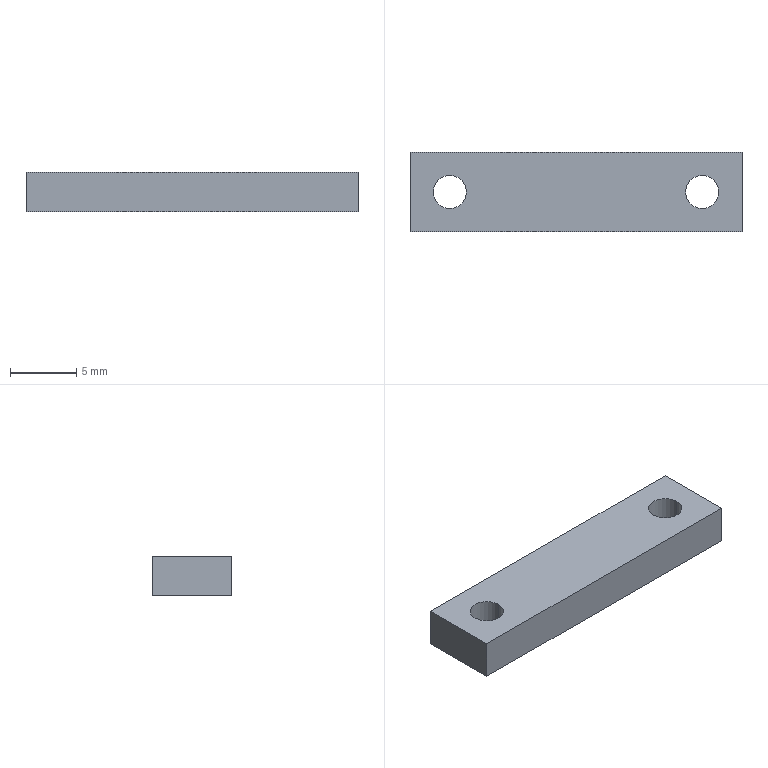Part | STEP file | 866-BDO024-93-11A | 1 solid | 10 faces | box 25 x 6 x 3 mm | volume 420.548 mm3 | plane 6 | cylinder 4 | commonest cylinder face diameters 2.5 x4
STEP:
#1=CARTESIAN_POINT('',(-10.75,0.,0.));
#2=VERTEX_POINT('',#1);
#3=CARTESIAN_POINT('',(-8.25,0.,0.));
#4=VERTEX_POINT('',#3);
#5=CARTESIAN_POINT('',(-9.5,0.,0.));
#6=DIRECTION('',(0.,0.,1.));
#7=DIRECTION('',(1.,0.,0.));
#8=AXIS2_PLACEMENT_3D('',#5,#6,#7);
#9=CIRCLE('',#8,1.25);
#10=EDGE_CURVE('',#2,#4,#9,.T.);
#11=ORIENTED_EDGE('',*,*,#10,.F.);
#12=CARTESIAN_POINT('',(-10.75,0.,3.));
#13=VERTEX_POINT('',#12);
#14=CARTESIAN_POINT('',(-10.75,0.,3.));
#15=DIRECTION('',(0.,0.,1.));
#16=VECTOR('',#15,1000.);
#17=LINE('',#14,#16);
#18=EDGE_CURVE('',#2,#13,#17,.T.);
#19=ORIENTED_EDGE('',*,*,#18,.T.);
#20=CARTESIAN_POINT('',(-8.25,0.,3.));
#21=VERTEX_POINT('',#20);
#22=CARTESIAN_POINT('',(-9.5,0.,3.));
#23=DIRECTION('',(0.,0.,1.));
#24=DIRECTION('',(1.,0.,0.));
#25=AXIS2_PLACEMENT_3D('',#22,#23,#24);
#26=CIRCLE('',#25,1.25);
#27=EDGE_CURVE('',#13,#21,#26,.T.);
#28=ORIENTED_EDGE('',*,*,#27,.T.);
#29=CARTESIAN_POINT('',(-8.25,0.,3.));
#30=DIRECTION('',(0.,0.,1.));
#31=VECTOR('',#30,1000.);
#32=LINE('',#29,#31);
#33=EDGE_CURVE('',#4,#21,#32,.T.);
#34=ORIENTED_EDGE('',*,*,#33,.F.);
#35=EDGE_LOOP('',(#11,#19,#28,#34));
#36=FACE_OUTER_BOUND('',#35,.T.);
#37=CARTESIAN_POINT('',(-9.5,0.,3.));
#38=DIRECTION('',(0.,0.,1.));
#39=DIRECTION('',(1.,0.,0.));
#40=AXIS2_PLACEMENT_3D('',#37,#38,#39);
#41=CYLINDRICAL_SURFACE('',#40,1.25);
#42=ADVANCED_FACE('',(#36),#41,.F.);
#43=CARTESIAN_POINT('',(8.25,0.,0.));
#44=VERTEX_POINT('',#43);
#45=CARTESIAN_POINT('',(10.75,0.,0.));
#46=VERTEX_POINT('',#45);
#47=CARTESIAN_POINT('',(9.5,0.,0.));
#48=DIRECTION('',(0.,0.,1.));
#49=DIRECTION('',(1.,0.,0.));
#50=AXIS2_PLACEMENT_3D('',#47,#48,#49);
#51=CIRCLE('',#50,1.25);
#52=EDGE_CURVE('',#44,#46,#51,.T.);
#53=ORIENTED_EDGE('',*,*,#52,.F.);
#54=CARTESIAN_POINT('',(8.25,0.,3.));
#55=VERTEX_POINT('',#54);
#56=CARTESIAN_POINT('',(8.25,0.,3.));
#57=DIRECTION('',(0.,0.,1.));
#58=VECTOR('',#57,1000.);
#59=LINE('',#56,#58);
#60=EDGE_CURVE('',#44,#55,#59,.T.);
#61=ORIENTED_EDGE('',*,*,#60,.T.);
#62=CARTESIAN_POINT('',(10.75,0.,3.));
#63=VERTEX_POINT('',#62);
#64=CARTESIAN_POINT('',(9.5,0.,3.));
#65=DIRECTION('',(0.,0.,1.));
#66=DIRECTION('',(1.,0.,0.));
#67=AXIS2_PLACEMENT_3D('',#64,#65,#66);
#68=CIRCLE('',#67,1.25);
#69=EDGE_CURVE('',#55,#63,#68,.T.);
#70=ORIENTED_EDGE('',*,*,#69,.T.);
#71=CARTESIAN_POINT('',(10.75,0.,3.));
#72=DIRECTION('',(0.,0.,1.));
#73=VECTOR('',#72,1000.);
#74=LINE('',#71,#73);
#75=EDGE_CURVE('',#46,#63,#74,.T.);
#76=ORIENTED_EDGE('',*,*,#75,.F.);
#77=EDGE_LOOP('',(#53,#61,#70,#76));
#78=FACE_OUTER_BOUND('',#77,.T.);
#79=CARTESIAN_POINT('',(9.5,0.,3.));
#80=DIRECTION('',(0.,0.,1.));
#81=DIRECTION('',(1.,0.,0.));
#82=AXIS2_PLACEMENT_3D('',#79,#80,#81);
#83=CYLINDRICAL_SURFACE('',#82,1.25);
#84=ADVANCED_FACE('',(#78),#83,.F.);
#85=CARTESIAN_POINT('',(-9.5,0.,3.));
#86=DIRECTION('',(0.,0.,1.));
#87=DIRECTION('',(1.,0.,0.));
#88=AXIS2_PLACEMENT_3D('',#85,#86,#87);
#89=CIRCLE('',#88,1.25);
#90=EDGE_CURVE('',#21,#13,#89,.T.);
#91=ORIENTED_EDGE('',*,*,#90,.F.);
#92=ORIENTED_EDGE('',*,*,#27,.F.);
#93=EDGE_LOOP('',(#91,#92));
#94=FACE_BOUND('',#93,.T.);
#95=CARTESIAN_POINT('',(12.5,-3.,3.));
#96=VERTEX_POINT('',#95);
#97=CARTESIAN_POINT('',(-12.5,-3.,3.));
#98=VERTEX_POINT('',#97);
#99=CARTESIAN_POINT('',(-12.5,-3.,3.));
#100=DIRECTION('',(-1.,0.,0.));
#101=VECTOR('',#100,1000.);
#102=LINE('',#99,#101);
#103=EDGE_CURVE('',#96,#98,#102,.T.);
#104=ORIENTED_EDGE('',*,*,#103,.F.);
#105=CARTESIAN_POINT('',(12.5,3.,3.));
#106=VERTEX_POINT('',#105);
#107=CARTESIAN_POINT('',(12.5,3.,3.));
#108=DIRECTION('',(0.,-1.,0.));
#109=VECTOR('',#108,1000.);
#110=LINE('',#107,#109);
#111=EDGE_CURVE('',#106,#96,#110,.T.);
#112=ORIENTED_EDGE('',*,*,#111,.F.);
#113=CARTESIAN_POINT('',(-12.5,3.,3.));
#114=VERTEX_POINT('',#113);
#115=CARTESIAN_POINT('',(-12.5,3.,3.));
#116=DIRECTION('',(1.,0.,0.));
#117=VECTOR('',#116,1000.);
#118=LINE('',#115,#117);
#119=EDGE_CURVE('',#114,#106,#118,.T.);
#120=ORIENTED_EDGE('',*,*,#119,.F.);
#121=CARTESIAN_POINT('',(-12.5,3.,3.));
#122=DIRECTION('',(0.,1.,0.));
#123=VECTOR('',#122,1000.);
#124=LINE('',#121,#123);
#125=EDGE_CURVE('',#98,#114,#124,.T.);
#126=ORIENTED_EDGE('',*,*,#125,.F.);
#127=EDGE_LOOP('',(#104,#112,#120,#126));
#128=FACE_OUTER_BOUND('',#127,.T.);
#129=CARTESIAN_POINT('',(9.5,0.,3.));
#130=DIRECTION('',(0.,0.,1.));
#131=DIRECTION('',(1.,0.,0.));
#132=AXIS2_PLACEMENT_3D('',#129,#130,#131);
#133=CIRCLE('',#132,1.25);
#134=EDGE_CURVE('',#63,#55,#133,.T.);
#135=ORIENTED_EDGE('',*,*,#134,.F.);
#136=ORIENTED_EDGE('',*,*,#69,.F.);
#137=EDGE_LOOP('',(#135,#136));
#138=FACE_BOUND('',#137,.T.);
#139=CARTESIAN_POINT('',(-12.5,3.,3.));
#140=DIRECTION('',(0.,0.,-1.));
#141=DIRECTION('',(-1.,0.,0.));
#142=AXIS2_PLACEMENT_3D('',#139,#140,#141);
#143=PLANE('',#142);
#144=ADVANCED_FACE('',(#94,#128,#138),#143,.F.);
#145=ORIENTED_EDGE('',*,*,#18,.F.);
#146=CARTESIAN_POINT('',(-9.5,0.,0.));
#147=DIRECTION('',(0.,0.,1.));
#148=DIRECTION('',(1.,0.,0.));
#149=AXIS2_PLACEMENT_3D('',#146,#147,#148);
#150=CIRCLE('',#149,1.25);
#151=EDGE_CURVE('',#4,#2,#150,.T.);
#152=ORIENTED_EDGE('',*,*,#151,.F.);
#153=ORIENTED_EDGE('',*,*,#33,.T.);
#154=ORIENTED_EDGE('',*,*,#90,.T.);
#155=EDGE_LOOP('',(#145,#152,#153,#154));
#156=FACE_OUTER_BOUND('',#155,.T.);
#157=CARTESIAN_POINT('',(-9.5,0.,3.));
#158=DIRECTION('',(0.,0.,1.));
#159=DIRECTION('',(1.,0.,0.));
#160=AXIS2_PLACEMENT_3D('',#157,#158,#159);
#161=CYLINDRICAL_SURFACE('',#160,1.25);
#162=ADVANCED_FACE('',(#156),#161,.F.);
#163=CARTESIAN_POINT('',(-12.5,-3.,0.));
#164=VERTEX_POINT('',#163);
#165=CARTESIAN_POINT('',(-12.5,-3.,3.));
#166=DIRECTION('',(0.,0.,-1.));
#167=VECTOR('',#166,1000.);
#168=LINE('',#165,#167);
#169=EDGE_CURVE('',#98,#164,#168,.T.);
#170=ORIENTED_EDGE('',*,*,#169,.F.);
#171=ORIENTED_EDGE('',*,*,#125,.T.);
#172=CARTESIAN_POINT('',(-12.5,3.,0.));
#173=VERTEX_POINT('',#172);
#174=CARTESIAN_POINT('',(-12.5,3.,3.));
#175=DIRECTION('',(0.,0.,1.));
#176=VECTOR('',#175,1000.);
#177=LINE('',#174,#176);
#178=EDGE_CURVE('',#173,#114,#177,.T.);
#179=ORIENTED_EDGE('',*,*,#178,.F.);
#180=CARTESIAN_POINT('',(-12.5,-3.,0.));
#181=DIRECTION('',(0.,1.,0.));
#182=VECTOR('',#181,1000.);
#183=LINE('',#180,#182);
#184=EDGE_CURVE('',#164,#173,#183,.T.);
#185=ORIENTED_EDGE('',*,*,#184,.F.);
#186=EDGE_LOOP('',(#170,#171,#179,#185));
#187=FACE_OUTER_BOUND('',#186,.T.);
#188=CARTESIAN_POINT('',(-12.5,-3.,3.));
#189=DIRECTION('',(1.,0.,0.));
#190=DIRECTION('',(0.,0.,-1.));
#191=AXIS2_PLACEMENT_3D('',#188,#189,#190);
#192=PLANE('',#191);
#193=ADVANCED_FACE('',(#187),#192,.F.);
#194=CARTESIAN_POINT('',(12.5,-3.,0.));
#195=VERTEX_POINT('',#194);
#196=CARTESIAN_POINT('',(12.5,-3.,3.));
#197=DIRECTION('',(0.,0.,-1.));
#198=VECTOR('',#197,1000.);
#199=LINE('',#196,#198);
#200=EDGE_CURVE('',#96,#195,#199,.T.);
#201=ORIENTED_EDGE('',*,*,#200,.F.);
#202=ORIENTED_EDGE('',*,*,#103,.T.);
#203=ORIENTED_EDGE('',*,*,#169,.T.);
#204=CARTESIAN_POINT('',(-12.5,-3.,0.));
#205=DIRECTION('',(-1.,0.,0.));
#206=VECTOR('',#205,1000.);
#207=LINE('',#204,#206);
#208=EDGE_CURVE('',#195,#164,#207,.T.);
#209=ORIENTED_EDGE('',*,*,#208,.F.);
#210=EDGE_LOOP('',(#201,#202,#203,#209));
#211=FACE_OUTER_BOUND('',#210,.T.);
#212=CARTESIAN_POINT('',(-12.5,-3.,3.));
#213=DIRECTION('',(0.,1.,0.));
#214=DIRECTION('',(0.,0.,1.));
#215=AXIS2_PLACEMENT_3D('',#212,#213,#214);
#216=PLANE('',#215);
#217=ADVANCED_FACE('',(#211),#216,.F.);
#218=CARTESIAN_POINT('',(12.5,3.,0.));
#219=VERTEX_POINT('',#218);
#220=CARTESIAN_POINT('',(12.5,3.,3.));
#221=DIRECTION('',(0.,0.,-1.));
#222=VECTOR('',#221,1000.);
#223=LINE('',#220,#222);
#224=EDGE_CURVE('',#106,#219,#223,.T.);
#225=ORIENTED_EDGE('',*,*,#224,.F.);
#226=ORIENTED_EDGE('',*,*,#111,.T.);
#227=ORIENTED_EDGE('',*,*,#200,.T.);
#228=CARTESIAN_POINT('',(12.5,-3.,0.));
#229=DIRECTION('',(0.,-1.,0.));
#230=VECTOR('',#229,1000.);
#231=LINE('',#228,#230);
#232=EDGE_CURVE('',#219,#195,#231,.T.);
#233=ORIENTED_EDGE('',*,*,#232,.F.);
#234=EDGE_LOOP('',(#225,#226,#227,#233));
#235=FACE_OUTER_BOUND('',#234,.T.);
#236=CARTESIAN_POINT('',(12.5,-3.,3.));
#237=DIRECTION('',(-1.,0.,0.));
#238=DIRECTION('',(0.,0.,1.));
#239=AXIS2_PLACEMENT_3D('',#236,#237,#238);
#240=PLANE('',#239);
#241=ADVANCED_FACE('',(#235),#240,.F.);
#242=ORIENTED_EDGE('',*,*,#178,.T.);
#243=ORIENTED_EDGE('',*,*,#119,.T.);
#244=ORIENTED_EDGE('',*,*,#224,.T.);
#245=CARTESIAN_POINT('',(-12.5,3.,0.));
#246=DIRECTION('',(1.,0.,0.));
#247=VECTOR('',#246,1000.);
#248=LINE('',#245,#247);
#249=EDGE_CURVE('',#173,#219,#248,.T.);
#250=ORIENTED_EDGE('',*,*,#249,.F.);
#251=EDGE_LOOP('',(#242,#243,#244,#250));
#252=FACE_OUTER_BOUND('',#251,.T.);
#253=CARTESIAN_POINT('',(-12.5,3.,3.));
#254=DIRECTION('',(0.,-1.,0.));
#255=DIRECTION('',(0.,0.,-1.));
#256=AXIS2_PLACEMENT_3D('',#253,#254,#255);
#257=PLANE('',#256);
#258=ADVANCED_FACE('',(#252),#257,.F.);
#259=ORIENTED_EDGE('',*,*,#60,.F.);
#260=CARTESIAN_POINT('',(9.5,0.,0.));
#261=DIRECTION('',(0.,0.,1.));
#262=DIRECTION('',(1.,0.,0.));
#263=AXIS2_PLACEMENT_3D('',#260,#261,#262);
#264=CIRCLE('',#263,1.25);
#265=EDGE_CURVE('',#46,#44,#264,.T.);
#266=ORIENTED_EDGE('',*,*,#265,.F.);
#267=ORIENTED_EDGE('',*,*,#75,.T.);
#268=ORIENTED_EDGE('',*,*,#134,.T.);
#269=EDGE_LOOP('',(#259,#266,#267,#268));
#270=FACE_OUTER_BOUND('',#269,.T.);
#271=CARTESIAN_POINT('',(9.5,0.,3.));
#272=DIRECTION('',(0.,0.,1.));
#273=DIRECTION('',(1.,0.,0.));
#274=AXIS2_PLACEMENT_3D('',#271,#272,#273);
#275=CYLINDRICAL_SURFACE('',#274,1.25);
#276=ADVANCED_FACE('',(#270),#275,.F.);
#277=ORIENTED_EDGE('',*,*,#232,.T.);
#278=ORIENTED_EDGE('',*,*,#208,.T.);
#279=ORIENTED_EDGE('',*,*,#184,.T.);
#280=ORIENTED_EDGE('',*,*,#249,.T.);
#281=EDGE_LOOP('',(#277,#278,#279,#280));
#282=FACE_OUTER_BOUND('',#281,.T.);
#283=ORIENTED_EDGE('',*,*,#265,.T.);
#284=ORIENTED_EDGE('',*,*,#52,.T.);
#285=EDGE_LOOP('',(#283,#284));
#286=FACE_BOUND('',#285,.T.);
#287=ORIENTED_EDGE('',*,*,#151,.T.);
#288=ORIENTED_EDGE('',*,*,#10,.T.);
#289=EDGE_LOOP('',(#287,#288));
#290=FACE_BOUND('',#289,.T.);
#291=CARTESIAN_POINT('',(-12.5,3.,0.));
#292=DIRECTION('',(0.,0.,-1.));
#293=DIRECTION('',(-1.,0.,0.));
#294=AXIS2_PLACEMENT_3D('',#291,#292,#293);
#295=PLANE('',#294);
#296=ADVANCED_FACE('',(#282,#286,#290),#295,.T.);
#297=CLOSED_SHELL('',(#42,#84,#144,#162,#193,#217,#241,#258,#276,#296));
#298=MANIFOLD_SOLID_BREP('',#297);
#299=CARTESIAN_POINT('',(0.,0.,0.));
#300=DIRECTION('',(0.,0.,1.));
#301=DIRECTION('',(1.,0.,0.));
#302=AXIS2_PLACEMENT_3D('',#299,#300,#301);
#303=(LENGTH_UNIT()NAMED_UNIT(*)SI_UNIT(.MILLI.,.METRE.));
#304=UNCERTAINTY_MEASURE_WITH_UNIT(LENGTH_MEASURE(0.00001),#303,'','');
#305=(NAMED_UNIT(*)PLANE_ANGLE_UNIT()SI_UNIT($,.RADIAN.));
#306=(NAMED_UNIT(*)SI_UNIT($,.STERADIAN.)SOLID_ANGLE_UNIT());
#307=(GEOMETRIC_REPRESENTATION_CONTEXT(3)GLOBAL_UNCERTAINTY_ASSIGNED_CONTEXT((#304))GLOBAL_UNIT_ASSIGNED_CONTEXT((#303,#305,#306))REPRESENTATION_CONTEXT('',''));
#308=ADVANCED_BREP_SHAPE_REPRESENTATION('',(#298,#302),#307);